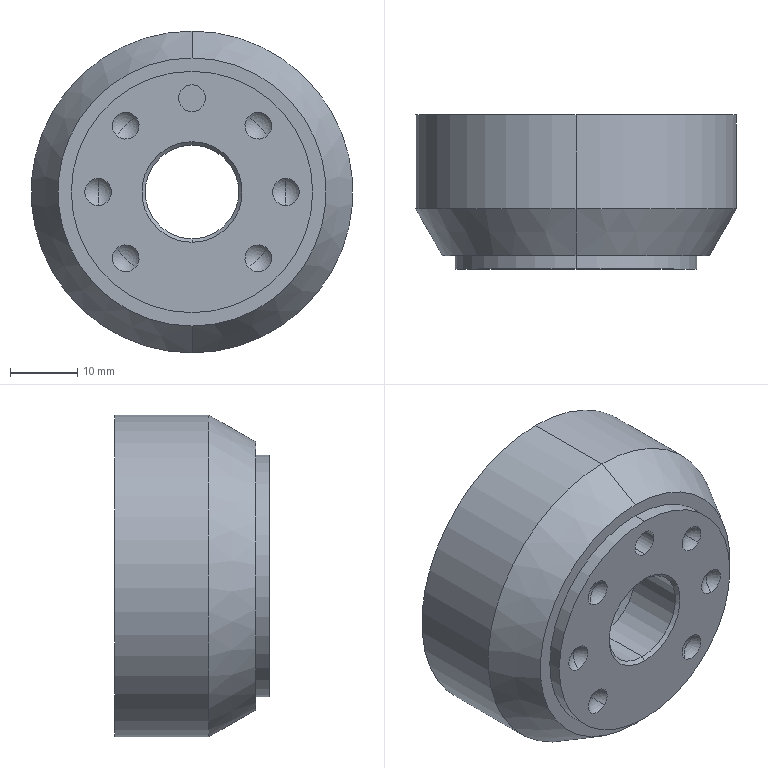Part | SolidWorks | features ICE 4, CirPattern 2, Chamfer 1, HoleWzd 1, RevCut 1, Revolution 1 | 1 solid | 58 faces | box 48 x 23 x 48 mm | volume 22097 mm3 | cone 20 | cylinder 20 | torus 12 | plane 6 | commonest cylinder face diameters 3.3 x8 4 x2 14 x2 18 x2 35 x2 36 x2
STEP:
#1=CARTESIAN_POINT('',(0.,0.5,7.));
#2=VERTEX_POINT('',#1);
#3=CARTESIAN_POINT('',(0.,0.5,-7.));
#4=VERTEX_POINT('',#3);
#5=CARTESIAN_POINT('',(0.,0.5,0.));
#6=DIRECTION('',(0.,-1.,0.));
#7=DIRECTION('',(0.,0.,-1.));
#8=AXIS2_PLACEMENT_3D('',#5,#6,#7);
#9=CIRCLE('',#8,7.);
#10=EDGE_CURVE('',#2,#4,#9,.T.);
#11=ORIENTED_EDGE('',*,*,#10,.F.);
#12=CARTESIAN_POINT('',(0.,0.,7.5));
#13=VERTEX_POINT('',#12);
#14=CARTESIAN_POINT('',(0.,0.,7.5));
#15=DIRECTION('',(0.,-0.7071,0.7071));
#16=VECTOR('',#15,1000.);
#17=LINE('',#14,#16);
#18=EDGE_CURVE('',#2,#13,#17,.T.);
#19=ORIENTED_EDGE('',*,*,#18,.T.);
#20=CARTESIAN_POINT('',(0.,0.,-7.5));
#21=VERTEX_POINT('',#20);
#22=CARTESIAN_POINT('',(0.,0.,0.));
#23=DIRECTION('',(0.,1.,0.));
#24=DIRECTION('',(0.,0.,-1.));
#25=AXIS2_PLACEMENT_3D('',#22,#23,#24);
#26=CIRCLE('',#25,7.5);
#27=EDGE_CURVE('',#21,#13,#26,.T.);
#28=ORIENTED_EDGE('',*,*,#27,.F.);
#29=CARTESIAN_POINT('',(0.,0.,-7.5));
#30=DIRECTION('',(0.,-0.7071,-0.7071));
#31=VECTOR('',#30,1000.);
#32=LINE('',#29,#31);
#33=EDGE_CURVE('',#4,#21,#32,.T.);
#34=ORIENTED_EDGE('',*,*,#33,.F.);
#35=EDGE_LOOP('',(#11,#19,#28,#34));
#36=FACE_OUTER_BOUND('',#35,.T.);
#37=CARTESIAN_POINT('',(0.,0.,0.));
#38=DIRECTION('',(0.,-1.,0.));
#39=DIRECTION('',(0.,0.,-1.));
#40=AXIS2_PLACEMENT_3D('',#37,#38,#39);
#41=CONICAL_SURFACE('',#40,7.5,0.7854);
#42=ADVANCED_FACE('',(#36),#41,.F.);
#43=CARTESIAN_POINT('',(20.75,22.625,-1.65));
#44=VERTEX_POINT('',#43);
#45=CARTESIAN_POINT('',(20.75,22.625,1.65));
#46=VERTEX_POINT('',#45);
#47=CARTESIAN_POINT('',(20.75,22.625,0.));
#48=DIRECTION('',(0.,1.,0.));
#49=DIRECTION('',(0.,0.,1.));
#50=AXIS2_PLACEMENT_3D('',#47,#48,#49);
#51=CIRCLE('',#50,1.65);
#52=EDGE_CURVE('',#44,#46,#51,.T.);
#53=ORIENTED_EDGE('',*,*,#52,.F.);
#54=CARTESIAN_POINT('',(20.75,23.,-2.025));
#55=VERTEX_POINT('',#54);
#56=CARTESIAN_POINT('',(20.75,23.,-2.025));
#57=DIRECTION('',(0.,0.7071,-0.7071));
#58=VECTOR('',#57,1000.);
#59=LINE('',#56,#58);
#60=EDGE_CURVE('',#44,#55,#59,.T.);
#61=ORIENTED_EDGE('',*,*,#60,.T.);
#62=CARTESIAN_POINT('',(20.75,23.,2.025));
#63=VERTEX_POINT('',#62);
#64=CARTESIAN_POINT('',(20.75,23.,0.));
#65=DIRECTION('',(0.,1.,0.));
#66=DIRECTION('',(0.,0.,1.));
#67=AXIS2_PLACEMENT_3D('',#64,#65,#66);
#68=CIRCLE('',#67,2.025);
#69=EDGE_CURVE('',#55,#63,#68,.T.);
#70=ORIENTED_EDGE('',*,*,#69,.T.);
#71=CARTESIAN_POINT('',(20.75,23.,2.025));
#72=DIRECTION('',(0.,0.7071,0.7071));
#73=VECTOR('',#72,1000.);
#74=LINE('',#71,#73);
#75=EDGE_CURVE('',#46,#63,#74,.T.);
#76=ORIENTED_EDGE('',*,*,#75,.F.);
#77=EDGE_LOOP('',(#53,#61,#70,#76));
#78=FACE_OUTER_BOUND('',#77,.T.);
#79=CARTESIAN_POINT('',(20.75,23.,0.));
#80=DIRECTION('',(0.,1.,0.));
#81=DIRECTION('',(0.,0.,1.));
#82=AXIS2_PLACEMENT_3D('',#79,#80,#81);
#83=CONICAL_SURFACE('',#82,2.025,0.7854);
#84=ADVANCED_FACE('',(#78),#83,.F.);
#85=CARTESIAN_POINT('',(20.75,15.,-1.65));
#86=VERTEX_POINT('',#85);
#87=CARTESIAN_POINT('',(20.75,15.,1.65));
#88=VERTEX_POINT('',#87);
#89=CARTESIAN_POINT('',(20.75,15.,0.));
#90=DIRECTION('',(0.,1.,0.));
#91=DIRECTION('',(0.,0.,1.));
#92=AXIS2_PLACEMENT_3D('',#89,#90,#91);
#93=CIRCLE('',#92,1.65);
#94=EDGE_CURVE('',#86,#88,#93,.T.);
#95=ORIENTED_EDGE('',*,*,#94,.F.);
#96=CARTESIAN_POINT('',(20.75,23.,-1.65));
#97=DIRECTION('',(0.,1.,0.));
#98=VECTOR('',#97,1000.);
#99=LINE('',#96,#98);
#100=EDGE_CURVE('',#86,#44,#99,.T.);
#101=ORIENTED_EDGE('',*,*,#100,.T.);
#102=ORIENTED_EDGE('',*,*,#52,.T.);
#103=CARTESIAN_POINT('',(20.75,23.,1.65));
#104=DIRECTION('',(0.,1.,0.));
#105=VECTOR('',#104,1000.);
#106=LINE('',#103,#105);
#107=EDGE_CURVE('',#88,#46,#106,.T.);
#108=ORIENTED_EDGE('',*,*,#107,.F.);
#109=EDGE_LOOP('',(#95,#101,#102,#108));
#110=FACE_OUTER_BOUND('',#109,.T.);
#111=CARTESIAN_POINT('',(20.75,23.,0.));
#112=DIRECTION('',(0.,1.,0.));
#113=DIRECTION('',(0.,0.,1.));
#114=AXIS2_PLACEMENT_3D('',#111,#112,#113);
#115=CYLINDRICAL_SURFACE('',#114,1.65);
#116=ADVANCED_FACE('',(#110),#115,.F.);
#117=CARTESIAN_POINT('',(20.75,14.009,0.));
#118=VERTEX_POINT('',#117);
#119=CARTESIAN_POINT('',(20.75,15.,1.65));
#120=DIRECTION('',(0.,0.515,0.8572));
#121=VECTOR('',#120,1000.);
#122=LINE('',#119,#121);
#123=EDGE_CURVE('',#118,#88,#122,.T.);
#124=ORIENTED_EDGE('',*,*,#123,.F.);
#125=CARTESIAN_POINT('',(20.75,15.,-1.65));
#126=DIRECTION('',(0.,0.515,-0.8572));
#127=VECTOR('',#126,1000.);
#128=LINE('',#125,#127);
#129=EDGE_CURVE('',#118,#86,#128,.T.);
#130=ORIENTED_EDGE('',*,*,#129,.T.);
#131=ORIENTED_EDGE('',*,*,#94,.T.);
#132=EDGE_LOOP('',(#124,#130,#131));
#133=FACE_OUTER_BOUND('',#132,.T.);
#134=CARTESIAN_POINT('',(20.75,15.,0.));
#135=DIRECTION('',(0.,1.,0.));
#136=DIRECTION('',(0.,0.,1.));
#137=AXIS2_PLACEMENT_3D('',#134,#135,#136);
#138=CONICAL_SURFACE('',#137,1.65,1.03);
#139=ADVANCED_FACE('',(#133),#138,.F.);
#140=CARTESIAN_POINT('',(0.,22.625,19.1));
#141=VERTEX_POINT('',#140);
#142=CARTESIAN_POINT('',(0.,22.625,22.4));
#143=VERTEX_POINT('',#142);
#144=CARTESIAN_POINT('',(0.,22.625,20.75));
#145=DIRECTION('',(0.,1.,0.));
#146=DIRECTION('',(0.,0.,1.));
#147=AXIS2_PLACEMENT_3D('',#144,#145,#146);
#148=CIRCLE('',#147,1.65);
#149=EDGE_CURVE('',#141,#143,#148,.T.);
#150=ORIENTED_EDGE('',*,*,#149,.F.);
#151=CARTESIAN_POINT('',(0.,23.,18.725));
#152=VERTEX_POINT('',#151);
#153=CARTESIAN_POINT('',(0.,23.,18.725));
#154=DIRECTION('',(0.,0.7071,-0.7071));
#155=VECTOR('',#154,1000.);
#156=LINE('',#153,#155);
#157=EDGE_CURVE('',#141,#152,#156,.T.);
#158=ORIENTED_EDGE('',*,*,#157,.T.);
#159=CARTESIAN_POINT('',(0.,23.,22.775));
#160=VERTEX_POINT('',#159);
#161=CARTESIAN_POINT('',(0.,23.,20.75));
#162=DIRECTION('',(0.,1.,0.));
#163=DIRECTION('',(0.,0.,1.));
#164=AXIS2_PLACEMENT_3D('',#161,#162,#163);
#165=CIRCLE('',#164,2.025);
#166=EDGE_CURVE('',#152,#160,#165,.T.);
#167=ORIENTED_EDGE('',*,*,#166,.T.);
#168=CARTESIAN_POINT('',(0.,23.,22.775));
#169=DIRECTION('',(0.,0.7071,0.7071));
#170=VECTOR('',#169,1000.);
#171=LINE('',#168,#170);
#172=EDGE_CURVE('',#143,#160,#171,.T.);
#173=ORIENTED_EDGE('',*,*,#172,.F.);
#174=EDGE_LOOP('',(#150,#158,#167,#173));
#175=FACE_OUTER_BOUND('',#174,.T.);
#176=CARTESIAN_POINT('',(0.,23.,20.75));
#177=DIRECTION('',(0.,1.,0.));
#178=DIRECTION('',(0.,0.,1.));
#179=AXIS2_PLACEMENT_3D('',#176,#177,#178);
#180=CONICAL_SURFACE('',#179,2.025,0.7854);
#181=ADVANCED_FACE('',(#175),#180,.F.);
#182=CARTESIAN_POINT('',(0.,15.,19.1));
#183=VERTEX_POINT('',#182);
#184=CARTESIAN_POINT('',(0.,15.,22.4));
#185=VERTEX_POINT('',#184);
#186=CARTESIAN_POINT('',(0.,15.,20.75));
#187=DIRECTION('',(0.,1.,0.));
#188=DIRECTION('',(0.,0.,1.));
#189=AXIS2_PLACEMENT_3D('',#186,#187,#188);
#190=CIRCLE('',#189,1.65);
#191=EDGE_CURVE('',#183,#185,#190,.T.);
#192=ORIENTED_EDGE('',*,*,#191,.F.);
#193=CARTESIAN_POINT('',(0.,23.,19.1));
#194=DIRECTION('',(0.,1.,0.));
#195=VECTOR('',#194,1000.);
#196=LINE('',#193,#195);
#197=EDGE_CURVE('',#183,#141,#196,.T.);
#198=ORIENTED_EDGE('',*,*,#197,.T.);
#199=ORIENTED_EDGE('',*,*,#149,.T.);
#200=CARTESIAN_POINT('',(0.,23.,22.4));
#201=DIRECTION('',(0.,1.,0.));
#202=VECTOR('',#201,1000.);
#203=LINE('',#200,#202);
#204=EDGE_CURVE('',#185,#143,#203,.T.);
#205=ORIENTED_EDGE('',*,*,#204,.F.);
#206=EDGE_LOOP('',(#192,#198,#199,#205));
#207=FACE_OUTER_BOUND('',#206,.T.);
#208=CARTESIAN_POINT('',(0.,23.,20.75));
#209=DIRECTION('',(0.,1.,0.));
#210=DIRECTION('',(0.,0.,1.));
#211=AXIS2_PLACEMENT_3D('',#208,#209,#210);
#212=CYLINDRICAL_SURFACE('',#211,1.65);
#213=ADVANCED_FACE('',(#207),#212,.F.);
#214=CARTESIAN_POINT('',(0.,14.009,20.75));
#215=VERTEX_POINT('',#214);
#216=CARTESIAN_POINT('',(0.,15.,22.4));
#217=DIRECTION('',(0.,0.515,0.8572));
#218=VECTOR('',#217,1000.);
#219=LINE('',#216,#218);
#220=EDGE_CURVE('',#215,#185,#219,.T.);
#221=ORIENTED_EDGE('',*,*,#220,.F.);
#222=CARTESIAN_POINT('',(0.,15.,19.1));
#223=DIRECTION('',(0.,0.515,-0.8572));
#224=VECTOR('',#223,1000.);
#225=LINE('',#222,#224);
#226=EDGE_CURVE('',#215,#183,#225,.T.);
#227=ORIENTED_EDGE('',*,*,#226,.T.);
#228=ORIENTED_EDGE('',*,*,#191,.T.);
#229=EDGE_LOOP('',(#221,#227,#228));
#230=FACE_OUTER_BOUND('',#229,.T.);
#231=CARTESIAN_POINT('',(0.,15.,20.75));
#232=DIRECTION('',(0.,1.,0.));
#233=DIRECTION('',(0.,0.,1.));
#234=AXIS2_PLACEMENT_3D('',#231,#232,#233);
#235=CONICAL_SURFACE('',#234,1.65,1.03);
#236=ADVANCED_FACE('',(#230),#235,.F.);
#237=CARTESIAN_POINT('',(-20.75,22.625,-1.65));
#238=VERTEX_POINT('',#237);
#239=CARTESIAN_POINT('',(-20.75,22.625,1.65));
#240=VERTEX_POINT('',#239);
#241=CARTESIAN_POINT('',(-20.75,22.625,0.));
#242=DIRECTION('',(0.,1.,0.));
#243=DIRECTION('',(0.,0.,1.));
#244=AXIS2_PLACEMENT_3D('',#241,#242,#243);
#245=CIRCLE('',#244,1.65);
#246=EDGE_CURVE('',#238,#240,#245,.T.);
#247=ORIENTED_EDGE('',*,*,#246,.F.);
#248=CARTESIAN_POINT('',(-20.75,23.,-2.025));
#249=VERTEX_POINT('',#248);
#250=CARTESIAN_POINT('',(-20.75,23.,-2.025));
#251=DIRECTION('',(0.,0.7071,-0.7071));
#252=VECTOR('',#251,1000.);
#253=LINE('',#250,#252);
#254=EDGE_CURVE('',#238,#249,#253,.T.);
#255=ORIENTED_EDGE('',*,*,#254,.T.);
#256=CARTESIAN_POINT('',(-20.75,23.,2.025));
#257=VERTEX_POINT('',#256);
#258=CARTESIAN_POINT('',(-20.75,23.,0.));
#259=DIRECTION('',(0.,1.,0.));
#260=DIRECTION('',(0.,0.,1.));
#261=AXIS2_PLACEMENT_3D('',#258,#259,#260);
#262=CIRCLE('',#261,2.025);
#263=EDGE_CURVE('',#249,#257,#262,.T.);
#264=ORIENTED_EDGE('',*,*,#263,.T.);
#265=CARTESIAN_POINT('',(-20.75,23.,2.025));
#266=DIRECTION('',(0.,0.7071,0.7071));
#267=VECTOR('',#266,1000.);
#268=LINE('',#265,#267);
#269=EDGE_CURVE('',#240,#257,#268,.T.);
#270=ORIENTED_EDGE('',*,*,#269,.F.);
#271=EDGE_LOOP('',(#247,#255,#264,#270));
#272=FACE_OUTER_BOUND('',#271,.T.);
#273=CARTESIAN_POINT('',(-20.75,23.,0.));
#274=DIRECTION('',(0.,1.,0.));
#275=DIRECTION('',(0.,0.,1.));
#276=AXIS2_PLACEMENT_3D('',#273,#274,#275);
#277=CONICAL_SURFACE('',#276,2.025,0.7854);
#278=ADVANCED_FACE('',(#272),#277,.F.);
#279=CARTESIAN_POINT('',(-20.75,15.,-1.65));
#280=VERTEX_POINT('',#279);
#281=CARTESIAN_POINT('',(-20.75,15.,1.65));
#282=VERTEX_POINT('',#281);
#283=CARTESIAN_POINT('',(-20.75,15.,0.));
#284=DIRECTION('',(0.,1.,0.));
#285=DIRECTION('',(0.,0.,1.));
#286=AXIS2_PLACEMENT_3D('',#283,#284,#285);
#287=CIRCLE('',#286,1.65);
#288=EDGE_CURVE('',#280,#282,#287,.T.);
#289=ORIENTED_EDGE('',*,*,#288,.F.);
#290=CARTESIAN_POINT('',(-20.75,23.,-1.65));
#291=DIRECTION('',(0.,1.,0.));
#292=VECTOR('',#291,1000.);
#293=LINE('',#290,#292);
#294=EDGE_CURVE('',#280,#238,#293,.T.);
#295=ORIENTED_EDGE('',*,*,#294,.T.);
#296=ORIENTED_EDGE('',*,*,#246,.T.);
#297=CARTESIAN_POINT('',(-20.75,23.,1.65));
#298=DIRECTION('',(0.,1.,0.));
#299=VECTOR('',#298,1000.);
#300=LINE('',#297,#299);
#301=EDGE_CURVE('',#282,#240,#300,.T.);
#302=ORIENTED_EDGE('',*,*,#301,.F.);
#303=EDGE_LOOP('',(#289,#295,#296,#302));
#304=FACE_OUTER_BOUND('',#303,.T.);
#305=CARTESIAN_POINT('',(-20.75,23.,0.));
#306=DIRECTION('',(0.,1.,0.));
#307=DIRECTION('',(0.,0.,1.));
#308=AXIS2_PLACEMENT_3D('',#305,#306,#307);
#309=CYLINDRICAL_SURFACE('',#308,1.65);
#310=ADVANCED_FACE('',(#304),#309,.F.);
#311=CARTESIAN_POINT('',(-20.75,14.009,0.));
#312=VERTEX_POINT('',#311);
#313=CARTESIAN_POINT('',(-20.75,15.,1.65));
#314=DIRECTION('',(0.,0.515,0.8572));
#315=VECTOR('',#314,1000.);
#316=LINE('',#313,#315);
#317=EDGE_CURVE('',#312,#282,#316,.T.);
#318=ORIENTED_EDGE('',*,*,#317,.F.);
#319=CARTESIAN_POINT('',(-20.75,15.,-1.65));
#320=DIRECTION('',(0.,0.515,-0.8572));
#321=VECTOR('',#320,1000.);
#322=LINE('',#319,#321);
#323=EDGE_CURVE('',#312,#280,#322,.T.);
#324=ORIENTED_EDGE('',*,*,#323,.T.);
#325=ORIENTED_EDGE('',*,*,#288,.T.);
#326=EDGE_LOOP('',(#318,#324,#325));
#327=FACE_OUTER_BOUND('',#326,.T.);
#328=CARTESIAN_POINT('',(-20.75,15.,0.));
#329=DIRECTION('',(0.,1.,0.));
#330=DIRECTION('',(0.,0.,1.));
#331=AXIS2_PLACEMENT_3D('',#328,#329,#330);
#332=CONICAL_SURFACE('',#331,1.65,1.03);
#333=ADVANCED_FACE('',(#327),#332,.F.);
#334=CARTESIAN_POINT('',(0.,22.625,-22.4));
#335=VERTEX_POINT('',#334);
#336=CARTESIAN_POINT('',(0.,22.625,-19.1));
#337=VERTEX_POINT('',#336);
#338=CARTESIAN_POINT('',(0.,22.625,-20.75));
#339=DIRECTION('',(0.,1.,0.));
#340=DIRECTION('',(0.,0.,1.));
#341=AXIS2_PLACEMENT_3D('',#338,#339,#340);
#342=CIRCLE('',#341,1.65);
#343=EDGE_CURVE('',#335,#337,#342,.T.);
#344=ORIENTED_EDGE('',*,*,#343,.F.);
#345=CARTESIAN_POINT('',(0.,23.,-22.775));
#346=VERTEX_POINT('',#345);
#347=CARTESIAN_POINT('',(0.,23.,-22.775));
#348=DIRECTION('',(0.,0.7071,-0.7071));
#349=VECTOR('',#348,1000.);
#350=LINE('',#347,#349);
#351=EDGE_CURVE('',#335,#346,#350,.T.);
#352=ORIENTED_EDGE('',*,*,#351,.T.);
#353=CARTESIAN_POINT('',(0.,23.,-18.725));
#354=VERTEX_POINT('',#353);
#355=CARTESIAN_POINT('',(0.,23.,-20.75));
#356=DIRECTION('',(0.,1.,0.));
#357=DIRECTION('',(0.,0.,1.));
#358=AXIS2_PLACEMENT_3D('',#355,#356,#357);
#359=CIRCLE('',#358,2.025);
#360=EDGE_CURVE('',#346,#354,#359,.T.);
#361=ORIENTED_EDGE('',*,*,#360,.T.);
#362=CARTESIAN_POINT('',(0.,23.,-18.725));
#363=DIRECTION('',(0.,0.7071,0.7071));
#364=VECTOR('',#363,1000.);
#365=LINE('',#362,#364);
#366=EDGE_CURVE('',#337,#354,#365,.T.);
#367=ORIENTED_EDGE('',*,*,#366,.F.);
#368=EDGE_LOOP('',(#344,#352,#361,#367));
#369=FACE_OUTER_BOUND('',#368,.T.);
#370=CARTESIAN_POINT('',(0.,23.,-20.75));
#371=DIRECTION('',(0.,1.,0.));
#372=DIRECTION('',(0.,0.,1.));
#373=AXIS2_PLACEMENT_3D('',#370,#371,#372);
#374=CONICAL_SURFACE('',#373,2.025,0.7854);
#375=ADVANCED_FACE('',(#369),#374,.F.);
#376=CARTESIAN_POINT('',(0.,15.,-22.4));
#377=VERTEX_POINT('',#376);
#378=CARTESIAN_POINT('',(0.,15.,-19.1));
#379=VERTEX_POINT('',#378);
#380=CARTESIAN_POINT('',(0.,15.,-20.75));
#381=DIRECTION('',(0.,1.,0.));
#382=DIRECTION('',(0.,0.,1.));
#383=AXIS2_PLACEMENT_3D('',#380,#381,#382);
#384=CIRCLE('',#383,1.65);
#385=EDGE_CURVE('',#377,#379,#384,.T.);
#386=ORIENTED_EDGE('',*,*,#385,.F.);
#387=CARTESIAN_POINT('',(0.,23.,-22.4));
#388=DIRECTION('',(0.,1.,0.));
#389=VECTOR('',#388,1000.);
#390=LINE('',#387,#389);
#391=EDGE_CURVE('',#377,#335,#390,.T.);
#392=ORIENTED_EDGE('',*,*,#391,.T.);
#393=ORIENTED_EDGE('',*,*,#343,.T.);
#394=CARTESIAN_POINT('',(0.,23.,-19.1));
#395=DIRECTION('',(0.,1.,0.));
#396=VECTOR('',#395,1000.);
#397=LINE('',#394,#396);
#398=EDGE_CURVE('',#379,#337,#397,.T.);
#399=ORIENTED_EDGE('',*,*,#398,.F.);
#400=EDGE_LOOP('',(#386,#392,#393,#399));
#401=FACE_OUTER_BOUND('',#400,.T.);
#402=CARTESIAN_POINT('',(0.,23.,-20.75));
#403=DIRECTION('',(0.,1.,0.));
#404=DIRECTION('',(0.,0.,1.));
#405=AXIS2_PLACEMENT_3D('',#402,#403,#404);
#406=CYLINDRICAL_SURFACE('',#405,1.65);
#407=ADVANCED_FACE('',(#401),#406,.F.);
#408=CARTESIAN_POINT('',(0.,14.009,-20.75));
#409=VERTEX_POINT('',#408);
#410=CARTESIAN_POINT('',(0.,15.,-19.1));
#411=DIRECTION('',(0.,0.515,0.8572));
#412=VECTOR('',#411,1000.);
#413=LINE('',#410,#412);
#414=EDGE_CURVE('',#409,#379,#413,.T.);
#415=ORIENTED_EDGE('',*,*,#414,.F.);
#416=CARTESIAN_POINT('',(0.,15.,-22.4));
#417=DIRECTION('',(0.,0.515,-0.8572));
#418=VECTOR('',#417,1000.);
#419=LINE('',#416,#418);
#420=EDGE_CURVE('',#409,#377,#419,.T.);
#421=ORIENTED_EDGE('',*,*,#420,.T.);
#422=ORIENTED_EDGE('',*,*,#385,.T.);
#423=EDGE_LOOP('',(#415,#421,#422));
#424=FACE_OUTER_BOUND('',#423,.T.);
#425=CARTESIAN_POINT('',(0.,15.,-20.75));
#426=DIRECTION('',(0.,1.,0.));
#427=DIRECTION('',(0.,0.,1.));
#428=AXIS2_PLACEMENT_3D('',#425,#426,#427);
#429=CONICAL_SURFACE('',#428,1.65,1.03);
#430=ADVANCED_FACE('',(#424),#429,.F.);
#431=CARTESIAN_POINT('',(-9.899,1.,-9.899));
#432=VERTEX_POINT('',#431);
#433=CARTESIAN_POINT('',(-8.485,0.,-11.314));
#434=VERTEX_POINT('',#433);
#435=CARTESIAN_POINT('',(-10.004,-1.796,-9.795));
#436=DIRECTION('',(-0.7071,0.,-0.7071));
#437=DIRECTION('',(-0.7071,0.,0.7071));
#438=AXIS2_PLACEMENT_3D('',#435,#436,#437);
#439=CIRCLE('',#438,2.8);
#440=EDGE_CURVE('',#432,#434,#439,.T.);
#441=ORIENTED_EDGE('',*,*,#440,.F.);
#442=CARTESIAN_POINT('',(-11.314,0.,-8.485));
#443=VERTEX_POINT('',#442);
#444=CARTESIAN_POINT('',(-9.795,-1.796,-10.004));
#445=DIRECTION('',(0.7071,0.,0.7071));
#446=DIRECTION('',(0.7071,0.,-0.7071));
#447=AXIS2_PLACEMENT_3D('',#444,#445,#446);
#448=CIRCLE('',#447,2.8);
#449=EDGE_CURVE('',#432,#443,#448,.T.);
#450=ORIENTED_EDGE('',*,*,#449,.T.);
#451=CARTESIAN_POINT('',(-9.899,0.,-9.899));
#452=DIRECTION('',(0.,-1.,0.));
#453=DIRECTION('',(0.7071,0.,-0.7071));
#454=AXIS2_PLACEMENT_3D('',#451,#452,#453);
#455=CIRCLE('',#454,2.);
#456=EDGE_CURVE('',#443,#434,#455,.T.);
#457=ORIENTED_EDGE('',*,*,#456,.T.);
#458=EDGE_LOOP('',(#441,#450,#457));
#459=FACE_OUTER_BOUND('',#458,.T.);
#460=CARTESIAN_POINT('',(-9.899,-1.796,-9.899));
#461=DIRECTION('',(0.,-1.,0.));
#462=DIRECTION('',(0.7071,0.,-0.7071));
#463=AXIS2_PLACEMENT_3D('',#460,#461,#462);
#464=TOROIDAL_SURFACE('',#463,-0.148,2.8);
#465=ADVANCED_FACE('',(#459),#464,.F.);
#466=CARTESIAN_POINT('',(9.899,1.,-9.899));
#467=VERTEX_POINT('',#466);
#468=CARTESIAN_POINT('',(11.314,0.,-8.485));
#469=VERTEX_POINT('',#468);
#470=CARTESIAN_POINT('',(9.795,-1.796,-10.004));
#471=DIRECTION('',(0.7071,0.,-0.7071));
#472=DIRECTION('',(-0.7071,0.,-0.7071));
#473=AXIS2_PLACEMENT_3D('',#470,#471,#472);
#474=CIRCLE('',#473,2.8);
#475=EDGE_CURVE('',#467,#469,#474,.T.);
#476=ORIENTED_EDGE('',*,*,#475,.F.);
#477=CARTESIAN_POINT('',(8.485,0.,-11.314));
#478=VERTEX_POINT('',#477);
#479=CARTESIAN_POINT('',(10.004,-1.796,-9.795));
#480=DIRECTION('',(-0.7071,0.,0.7071));
#481=DIRECTION('',(0.7071,0.,0.7071));
#482=AXIS2_PLACEMENT_3D('',#479,#480,#481);
#483=CIRCLE('',#482,2.8);
#484=EDGE_CURVE('',#467,#478,#483,.T.);
#485=ORIENTED_EDGE('',*,*,#484,.T.);
#486=CARTESIAN_POINT('',(9.899,0.,-9.899));
#487=DIRECTION('',(0.,-1.,0.));
#488=DIRECTION('',(0.7071,0.,0.7071));
#489=AXIS2_PLACEMENT_3D('',#486,#487,#488);
#490=CIRCLE('',#489,2.);
#491=EDGE_CURVE('',#478,#469,#490,.T.);
#492=ORIENTED_EDGE('',*,*,#491,.T.);
#493=EDGE_LOOP('',(#476,#485,#492));
#494=FACE_OUTER_BOUND('',#493,.T.);
#495=CARTESIAN_POINT('',(9.899,-1.796,-9.899));
#496=DIRECTION('',(0.,-1.,0.));
#497=DIRECTION('',(0.7071,0.,0.7071));
#498=AXIS2_PLACEMENT_3D('',#495,#496,#497);
#499=TOROIDAL_SURFACE('',#498,-0.148,2.8);
#500=ADVANCED_FACE('',(#494),#499,.F.);
#501=CARTESIAN_POINT('',(14.,1.,0.));
#502=VERTEX_POINT('',#501);
#503=CARTESIAN_POINT('',(14.,0.,2.));
#504=VERTEX_POINT('',#503);
#505=CARTESIAN_POINT('',(14.,-1.796,-0.148));
#506=DIRECTION('',(1.,0.,0.));
#507=DIRECTION('',(0.,0.,-1.));
#508=AXIS2_PLACEMENT_3D('',#505,#506,#507);
#509=CIRCLE('',#508,2.8);
#510=EDGE_CURVE('',#502,#504,#509,.T.);
#511=ORIENTED_EDGE('',*,*,#510,.F.);
#512=CARTESIAN_POINT('',(14.,0.,-2.));
#513=VERTEX_POINT('',#512);
#514=CARTESIAN_POINT('',(14.,-1.796,0.148));
#515=DIRECTION('',(-1.,0.,0.));
#516=DIRECTION('',(0.,0.,1.));
#517=AXIS2_PLACEMENT_3D('',#514,#515,#516);
#518=CIRCLE('',#517,2.8);
#519=EDGE_CURVE('',#502,#513,#518,.T.);
#520=ORIENTED_EDGE('',*,*,#519,.T.);
#521=CARTESIAN_POINT('',(14.,0.,0.));
#522=DIRECTION('',(0.,-1.,0.));
#523=DIRECTION('',(0.,0.,1.));
#524=AXIS2_PLACEMENT_3D('',#521,#522,#523);
#525=CIRCLE('',#524,2.);
#526=EDGE_CURVE('',#513,#504,#525,.T.);
#527=ORIENTED_EDGE('',*,*,#526,.T.);
#528=EDGE_LOOP('',(#511,#520,#527));
#529=FACE_OUTER_BOUND('',#528,.T.);
#530=CARTESIAN_POINT('',(14.,-1.796,0.));
#531=DIRECTION('',(0.,-1.,0.));
#532=DIRECTION('',(0.,0.,1.));
#533=AXIS2_PLACEMENT_3D('',#530,#531,#532);
#534=TOROIDAL_SURFACE('',#533,-0.148,2.8);
#535=ADVANCED_FACE('',(#529),#534,.F.);
#536=CARTESIAN_POINT('',(9.899,1.,9.899));
#537=VERTEX_POINT('',#536);
#538=CARTESIAN_POINT('',(8.485,0.,11.314));
#539=VERTEX_POINT('',#538);
#540=CARTESIAN_POINT('',(10.004,-1.796,9.795));
#541=DIRECTION('',(0.7071,0.,0.7071));
#542=DIRECTION('',(0.7071,0.,-0.7071));
#543=AXIS2_PLACEMENT_3D('',#540,#541,#542);
#544=CIRCLE('',#543,2.8);
#545=EDGE_CURVE('',#537,#539,#544,.T.);
#546=ORIENTED_EDGE('',*,*,#545,.F.);
#547=CARTESIAN_POINT('',(11.314,0.,8.485));
#548=VERTEX_POINT('',#547);
#549=CARTESIAN_POINT('',(9.795,-1.796,10.004));
#550=DIRECTION('',(-0.7071,0.,-0.7071));
#551=DIRECTION('',(-0.7071,0.,0.7071));
#552=AXIS2_PLACEMENT_3D('',#549,#550,#551);
#553=CIRCLE('',#552,2.8);
#554=EDGE_CURVE('',#537,#548,#553,.T.);
#555=ORIENTED_EDGE('',*,*,#554,.T.);
#556=CARTESIAN_POINT('',(9.899,0.,9.899));
#557=DIRECTION('',(0.,-1.,0.));
#558=DIRECTION('',(-0.7071,0.,0.7071));
#559=AXIS2_PLACEMENT_3D('',#556,#557,#558);
#560=CIRCLE('',#559,2.);
#561=EDGE_CURVE('',#548,#539,#560,.T.);
#562=ORIENTED_EDGE('',*,*,#561,.T.);
#563=EDGE_LOOP('',(#546,#555,#562));
#564=FACE_OUTER_BOUND('',#563,.T.);
#565=CARTESIAN_POINT('',(9.899,-1.796,9.899));
#566=DIRECTION('',(0.,-1.,0.));
#567=DIRECTION('',(-0.7071,0.,0.7071));
#568=AXIS2_PLACEMENT_3D('',#565,#566,#567);
#569=TOROIDAL_SURFACE('',#568,-0.148,2.8);
#570=ADVANCED_FACE('',(#564),#569,.F.);
#571=CARTESIAN_POINT('',(-9.899,1.,9.899));
#572=VERTEX_POINT('',#571);
#573=CARTESIAN_POINT('',(-11.314,0.,8.485));
#574=VERTEX_POINT('',#573);
#575=CARTESIAN_POINT('',(-9.795,-1.796,10.004));
#576=DIRECTION('',(-0.7071,0.,0.7071));
#577=DIRECTION('',(0.7071,0.,0.7071));
#578=AXIS2_PLACEMENT_3D('',#575,#576,#577);
#579=CIRCLE('',#578,2.8);
#580=EDGE_CURVE('',#572,#574,#579,.T.);
#581=ORIENTED_EDGE('',*,*,#580,.F.);
#582=CARTESIAN_POINT('',(-8.485,0.,11.314));
#583=VERTEX_POINT('',#582);
#584=CARTESIAN_POINT('',(-10.004,-1.796,9.795));
#585=DIRECTION('',(0.7071,0.,-0.7071));
#586=DIRECTION('',(-0.7071,0.,-0.7071));
#587=AXIS2_PLACEMENT_3D('',#584,#585,#586);
#588=CIRCLE('',#587,2.8);
#589=EDGE_CURVE('',#572,#583,#588,.T.);
#590=ORIENTED_EDGE('',*,*,#589,.T.);
#591=CARTESIAN_POINT('',(-9.899,0.,9.899));
#592=DIRECTION('',(0.,-1.,0.));
#593=DIRECTION('',(-0.7071,0.,-0.7071));
#594=AXIS2_PLACEMENT_3D('',#591,#592,#593);
#595=CIRCLE('',#594,2.);
#596=EDGE_CURVE('',#583,#574,#595,.T.);
#597=ORIENTED_EDGE('',*,*,#596,.T.);
#598=EDGE_LOOP('',(#581,#590,#597));
#599=FACE_OUTER_BOUND('',#598,.T.);
#600=CARTESIAN_POINT('',(-9.899,-1.796,9.899));
#601=DIRECTION('',(0.,-1.,0.));
#602=DIRECTION('',(-0.7071,0.,-0.7071));
#603=AXIS2_PLACEMENT_3D('',#600,#601,#602);
#604=TOROIDAL_SURFACE('',#603,-0.148,2.8);
#605=ADVANCED_FACE('',(#599),#604,.F.);
#606=CARTESIAN_POINT('',(-14.,1.,0.));
#607=VERTEX_POINT('',#606);
#608=CARTESIAN_POINT('',(-14.,0.,-2.));
#609=VERTEX_POINT('',#608);
#610=CARTESIAN_POINT('',(-14.,-1.796,0.148));
#611=DIRECTION('',(-1.,0.,0.));
#612=DIRECTION('',(0.,0.,1.));
#613=AXIS2_PLACEMENT_3D('',#610,#611,#612);
#614=CIRCLE('',#613,2.8);
#615=EDGE_CURVE('',#607,#609,#614,.T.);
#616=ORIENTED_EDGE('',*,*,#615,.F.);
#617=CARTESIAN_POINT('',(-14.,0.,2.));
#618=VERTEX_POINT('',#617);
#619=CARTESIAN_POINT('',(-14.,-1.796,-0.148));
#620=DIRECTION('',(1.,0.,0.));
#621=DIRECTION('',(0.,0.,-1.));
#622=AXIS2_PLACEMENT_3D('',#619,#620,#621);
#623=CIRCLE('',#622,2.8);
#624=EDGE_CURVE('',#607,#618,#623,.T.);
#625=ORIENTED_EDGE('',*,*,#624,.T.);
#626=CARTESIAN_POINT('',(-14.,0.,0.));
#627=DIRECTION('',(0.,-1.,0.));
#628=DIRECTION('',(0.,0.,-1.));
#629=AXIS2_PLACEMENT_3D('',#626,#627,#628);
#630=CIRCLE('',#629,2.);
#631=EDGE_CURVE('',#618,#609,#630,.T.);
#632=ORIENTED_EDGE('',*,*,#631,.T.);
#633=EDGE_LOOP('',(#616,#625,#632));
#634=FACE_OUTER_BOUND('',#633,.T.);
#635=CARTESIAN_POINT('',(-14.,-1.796,0.));
#636=DIRECTION('',(0.,-1.,0.));
#637=DIRECTION('',(0.,0.,-1.));
#638=AXIS2_PLACEMENT_3D('',#635,#636,#637);
#639=TOROIDAL_SURFACE('',#638,-0.148,2.8);
#640=ADVANCED_FACE('',(#634),#639,.F.);
#641=CARTESIAN_POINT('',(0.,4.,16.));
#642=VERTEX_POINT('',#641);
#643=CARTESIAN_POINT('',(0.,4.,12.));
#644=VERTEX_POINT('',#643);
#645=CARTESIAN_POINT('',(0.,4.,14.));
#646=DIRECTION('',(0.,-1.,0.));
#647=DIRECTION('',(0.,0.,-1.));
#648=AXIS2_PLACEMENT_3D('',#645,#646,#647);
#649=CIRCLE('',#648,2.);
#650=EDGE_CURVE('',#642,#644,#649,.T.);
#651=ORIENTED_EDGE('',*,*,#650,.F.);
#652=CARTESIAN_POINT('',(0.,0.,16.));
#653=VERTEX_POINT('',#652);
#654=CARTESIAN_POINT('',(0.,4.,16.));
#655=DIRECTION('',(0.,-1.,0.));
#656=VECTOR('',#655,1000.);
#657=LINE('',#654,#656);
#658=EDGE_CURVE('',#642,#653,#657,.T.);
#659=ORIENTED_EDGE('',*,*,#658,.T.);
#660=CARTESIAN_POINT('',(0.,0.,12.));
#661=VERTEX_POINT('',#660);
#662=CARTESIAN_POINT('',(0.,0.,14.));
#663=DIRECTION('',(0.,-1.,0.));
#664=DIRECTION('',(0.,0.,-1.));
#665=AXIS2_PLACEMENT_3D('',#662,#663,#664);
#666=CIRCLE('',#665,2.);
#667=EDGE_CURVE('',#653,#661,#666,.T.);
#668=ORIENTED_EDGE('',*,*,#667,.T.);
#669=CARTESIAN_POINT('',(0.,4.,12.));
#670=DIRECTION('',(0.,-1.,0.));
#671=VECTOR('',#670,1000.);
#672=LINE('',#669,#671);
#673=EDGE_CURVE('',#644,#661,#672,.T.);
#674=ORIENTED_EDGE('',*,*,#673,.F.);
#675=EDGE_LOOP('',(#651,#659,#668,#674));
#676=FACE_OUTER_BOUND('',#675,.T.);
#677=CARTESIAN_POINT('',(0.,4.,14.));
#678=DIRECTION('',(0.,-1.,0.));
#679=DIRECTION('',(0.,0.,-1.));
#680=AXIS2_PLACEMENT_3D('',#677,#678,#679);
#681=CYLINDRICAL_SURFACE('',#680,2.);
#682=ADVANCED_FACE('',(#676),#681,.F.);
#683=ORIENTED_EDGE('',*,*,#10,.T.);
#684=CARTESIAN_POINT('',(0.,9.,-7.));
#685=VERTEX_POINT('',#684);
#686=CARTESIAN_POINT('',(0.,0.,-7.));
#687=DIRECTION('',(0.,1.,0.));
#688=VECTOR('',#687,1000.);
#689=LINE('',#686,#688);
#690=EDGE_CURVE('',#4,#685,#689,.T.);
#691=ORIENTED_EDGE('',*,*,#690,.T.);
#692=CARTESIAN_POINT('',(0.,9.,7.));
#693=VERTEX_POINT('',#692);
#694=CARTESIAN_POINT('',(0.,9.,0.));
#695=DIRECTION('',(0.,1.,0.));
#696=DIRECTION('',(0.,0.,1.));
#697=AXIS2_PLACEMENT_3D('',#694,#695,#696);
#698=CIRCLE('',#697,7.);
#699=EDGE_CURVE('',#685,#693,#698,.T.);
#700=ORIENTED_EDGE('',*,*,#699,.T.);
#701=CARTESIAN_POINT('',(0.,0.,7.));
#702=DIRECTION('',(0.,1.,0.));
#703=VECTOR('',#702,1000.);
#704=LINE('',#701,#703);
#705=EDGE_CURVE('',#2,#693,#704,.T.);
#706=ORIENTED_EDGE('',*,*,#705,.F.);
#707=EDGE_LOOP('',(#683,#691,#700,#706));
#708=FACE_OUTER_BOUND('',#707,.T.);
#709=CARTESIAN_POINT('',(0.,0.,0.));
#710=DIRECTION('',(0.,1.,0.));
#711=DIRECTION('',(0.,0.,1.));
#712=AXIS2_PLACEMENT_3D('',#709,#710,#711);
#713=CYLINDRICAL_SURFACE('',#712,7.);
#714=ADVANCED_FACE('',(#708),#713,.F.);
#715=CARTESIAN_POINT('',(0.,9.,9.));
#716=VERTEX_POINT('',#715);
#717=CARTESIAN_POINT('',(0.,9.,-9.));
#718=VERTEX_POINT('',#717);
#719=CARTESIAN_POINT('',(0.,9.,0.));
#720=DIRECTION('',(0.,1.,0.));
#721=DIRECTION('',(0.,0.,1.));
#722=AXIS2_PLACEMENT_3D('',#719,#720,#721);
#723=CIRCLE('',#722,9.);
#724=EDGE_CURVE('',#716,#718,#723,.T.);
#725=ORIENTED_EDGE('',*,*,#724,.F.);
#726=CARTESIAN_POINT('',(0.,8.,9.));
#727=VERTEX_POINT('',#726);
#728=CARTESIAN_POINT('',(0.,9.,9.));
#729=DIRECTION('',(0.,-1.,0.));
#730=VECTOR('',#729,1000.);
#731=LINE('',#728,#730);
#732=EDGE_CURVE('',#716,#727,#731,.T.);
#733=ORIENTED_EDGE('',*,*,#732,.T.);
#734=CARTESIAN_POINT('',(0.,8.,-9.));
#735=VERTEX_POINT('',#734);
#736=CARTESIAN_POINT('',(0.,8.,0.));
#737=DIRECTION('',(0.,1.,0.));
#738=DIRECTION('',(0.,0.,1.));
#739=AXIS2_PLACEMENT_3D('',#736,#737,#738);
#740=CIRCLE('',#739,9.);
#741=EDGE_CURVE('',#727,#735,#740,.T.);
#742=ORIENTED_EDGE('',*,*,#741,.T.);
#743=CARTESIAN_POINT('',(0.,9.,-9.));
#744=DIRECTION('',(0.,-1.,0.));
#745=VECTOR('',#744,1000.);
#746=LINE('',#743,#745);
#747=EDGE_CURVE('',#718,#735,#746,.T.);
#748=ORIENTED_EDGE('',*,*,#747,.F.);
#749=EDGE_LOOP('',(#725,#733,#742,#748));
#750=FACE_OUTER_BOUND('',#749,.T.);
#751=CARTESIAN_POINT('',(0.,9.,0.));
#752=DIRECTION('',(0.,-1.,0.));
#753=DIRECTION('',(0.,0.,-1.));
#754=AXIS2_PLACEMENT_3D('',#751,#752,#753);
#755=CYLINDRICAL_SURFACE('',#754,9.);
#756=ADVANCED_FACE('',(#750),#755,.T.);
#757=CARTESIAN_POINT('',(0.,8.,-17.5));
#758=VERTEX_POINT('',#757);
#759=CARTESIAN_POINT('',(0.,8.,17.5));
#760=VERTEX_POINT('',#759);
#761=CARTESIAN_POINT('',(0.,8.,0.));
#762=DIRECTION('',(0.,1.,0.));
#763=DIRECTION('',(0.,0.,1.));
#764=AXIS2_PLACEMENT_3D('',#761,#762,#763);
#765=CIRCLE('',#764,17.5);
#766=EDGE_CURVE('',#758,#760,#765,.T.);
#767=ORIENTED_EDGE('',*,*,#766,.F.);
#768=CARTESIAN_POINT('',(0.,23.,-17.5));
#769=VERTEX_POINT('',#768);
#770=CARTESIAN_POINT('',(0.,8.,-17.5));
#771=DIRECTION('',(0.,1.,0.));
#772=VECTOR('',#771,1000.);
#773=LINE('',#770,#772);
#774=EDGE_CURVE('',#758,#769,#773,.T.);
#775=ORIENTED_EDGE('',*,*,#774,.T.);
#776=CARTESIAN_POINT('',(0.,23.,17.5));
#777=VERTEX_POINT('',#776);
#778=CARTESIAN_POINT('',(0.,23.,0.));
#779=DIRECTION('',(0.,1.,0.));
#780=DIRECTION('',(0.,0.,1.));
#781=AXIS2_PLACEMENT_3D('',#778,#779,#780);
#782=CIRCLE('',#781,17.5);
#783=EDGE_CURVE('',#769,#777,#782,.T.);
#784=ORIENTED_EDGE('',*,*,#783,.T.);
#785=CARTESIAN_POINT('',(0.,8.,17.5));
#786=DIRECTION('',(0.,1.,0.));
#787=VECTOR('',#786,1000.);
#788=LINE('',#785,#787);
#789=EDGE_CURVE('',#760,#777,#788,.T.);
#790=ORIENTED_EDGE('',*,*,#789,.F.);
#791=EDGE_LOOP('',(#767,#775,#784,#790));
#792=FACE_OUTER_BOUND('',#791,.T.);
#793=CARTESIAN_POINT('',(0.,8.,0.));
#794=DIRECTION('',(0.,1.,0.));
#795=DIRECTION('',(0.,0.,1.));
#796=AXIS2_PLACEMENT_3D('',#793,#794,#795);
#797=CYLINDRICAL_SURFACE('',#796,17.5);
#798=ADVANCED_FACE('',(#792),#797,.F.);
#799=CARTESIAN_POINT('',(0.,9.,24.));
#800=VERTEX_POINT('',#799);
#801=CARTESIAN_POINT('',(0.,9.,-24.));
#802=VERTEX_POINT('',#801);
#803=CARTESIAN_POINT('',(0.,9.,0.));
#804=DIRECTION('',(0.,1.,0.));
#805=DIRECTION('',(0.,0.,1.));
#806=AXIS2_PLACEMENT_3D('',#803,#804,#805);
#807=CIRCLE('',#806,24.);
#808=EDGE_CURVE('',#800,#802,#807,.T.);
#809=ORIENTED_EDGE('',*,*,#808,.T.);
#810=CARTESIAN_POINT('',(0.,23.,-24.));
#811=VERTEX_POINT('',#810);
#812=CARTESIAN_POINT('',(0.,23.,-24.));
#813=DIRECTION('',(0.,1.,0.));
#814=VECTOR('',#813,1000.);
#815=LINE('',#812,#814);
#816=EDGE_CURVE('',#802,#811,#815,.T.);
#817=ORIENTED_EDGE('',*,*,#816,.T.);
#818=CARTESIAN_POINT('',(0.,23.,24.));
#819=VERTEX_POINT('',#818);
#820=CARTESIAN_POINT('',(0.,23.,0.));
#821=DIRECTION('',(0.,1.,0.));
#822=DIRECTION('',(0.,0.,1.));
#823=AXIS2_PLACEMENT_3D('',#820,#821,#822);
#824=CIRCLE('',#823,24.);
#825=EDGE_CURVE('',#819,#811,#824,.T.);
#826=ORIENTED_EDGE('',*,*,#825,.F.);
#827=CARTESIAN_POINT('',(0.,23.,24.));
#828=DIRECTION('',(0.,1.,0.));
#829=VECTOR('',#828,1000.);
#830=LINE('',#827,#829);
#831=EDGE_CURVE('',#800,#819,#830,.T.);
#832=ORIENTED_EDGE('',*,*,#831,.F.);
#833=EDGE_LOOP('',(#809,#817,#826,#832));
#834=FACE_OUTER_BOUND('',#833,.T.);
#835=CARTESIAN_POINT('',(0.,23.,0.));
#836=DIRECTION('',(0.,1.,0.));
#837=DIRECTION('',(0.,0.,1.));
#838=AXIS2_PLACEMENT_3D('',#835,#836,#837);
#839=CYLINDRICAL_SURFACE('',#838,24.);
#840=ADVANCED_FACE('',(#834),#839,.T.);
#841=CARTESIAN_POINT('',(0.,2.,20.));
#842=VERTEX_POINT('',#841);
#843=CARTESIAN_POINT('',(0.,2.,-20.));
#844=VERTEX_POINT('',#843);
#845=CARTESIAN_POINT('',(0.,2.,0.));
#846=DIRECTION('',(0.,1.,0.));
#847=DIRECTION('',(0.,0.,1.));
#848=AXIS2_PLACEMENT_3D('',#845,#846,#847);
#849=CIRCLE('',#848,20.);
#850=EDGE_CURVE('',#842,#844,#849,.T.);
#851=ORIENTED_EDGE('',*,*,#850,.T.);
#852=CARTESIAN_POINT('',(0.,9.,-24.));
#853=DIRECTION('',(0.,0.8682,-0.4961));
#854=VECTOR('',#853,1000.);
#855=LINE('',#852,#854);
#856=EDGE_CURVE('',#844,#802,#855,.T.);
#857=ORIENTED_EDGE('',*,*,#856,.T.);
#858=ORIENTED_EDGE('',*,*,#808,.F.);
#859=CARTESIAN_POINT('',(0.,9.,24.));
#860=DIRECTION('',(0.,0.8682,0.4961));
#861=VECTOR('',#860,1000.);
#862=LINE('',#859,#861);
#863=EDGE_CURVE('',#842,#800,#862,.T.);
#864=ORIENTED_EDGE('',*,*,#863,.F.);
#865=EDGE_LOOP('',(#851,#857,#858,#864));
#866=FACE_OUTER_BOUND('',#865,.T.);
#867=CARTESIAN_POINT('',(0.,9.,0.));
#868=DIRECTION('',(0.,1.,0.));
#869=DIRECTION('',(0.,0.,1.));
#870=AXIS2_PLACEMENT_3D('',#867,#868,#869);
#871=CONICAL_SURFACE('',#870,24.,0.5191);
#872=ADVANCED_FACE('',(#866),#871,.T.);
#873=CARTESIAN_POINT('',(0.,0.,18.));
#874=VERTEX_POINT('',#873);
#875=CARTESIAN_POINT('',(0.,0.,-18.));
#876=VERTEX_POINT('',#875);
#877=CARTESIAN_POINT('',(0.,0.,0.));
#878=DIRECTION('',(0.,1.,0.));
#879=DIRECTION('',(0.,0.,1.));
#880=AXIS2_PLACEMENT_3D('',#877,#878,#879);
#881=CIRCLE('',#880,18.);
#882=EDGE_CURVE('',#874,#876,#881,.T.);
#883=ORIENTED_EDGE('',*,*,#882,.T.);
#884=CARTESIAN_POINT('',(0.,2.,-18.));
#885=VERTEX_POINT('',#884);
#886=CARTESIAN_POINT('',(0.,23.,-18.));
#887=DIRECTION('',(0.,1.,0.));
#888=VECTOR('',#887,1000.);
#889=LINE('',#886,#888);
#890=EDGE_CURVE('',#876,#885,#889,.T.);
#891=ORIENTED_EDGE('',*,*,#890,.T.);
#892=CARTESIAN_POINT('',(0.,2.,18.));
#893=VERTEX_POINT('',#892);
#894=CARTESIAN_POINT('',(0.,2.,0.));
#895=DIRECTION('',(0.,1.,0.));
#896=DIRECTION('',(0.,0.,1.));
#897=AXIS2_PLACEMENT_3D('',#894,#895,#896);
#898=CIRCLE('',#897,18.);
#899=EDGE_CURVE('',#893,#885,#898,.T.);
#900=ORIENTED_EDGE('',*,*,#899,.F.);
#901=CARTESIAN_POINT('',(0.,23.,18.));
#902=DIRECTION('',(0.,1.,0.));
#903=VECTOR('',#902,1000.);
#904=LINE('',#901,#903);
#905=EDGE_CURVE('',#874,#893,#904,.T.);
#906=ORIENTED_EDGE('',*,*,#905,.F.);
#907=EDGE_LOOP('',(#883,#891,#900,#906));
#908=FACE_OUTER_BOUND('',#907,.T.);
#909=CARTESIAN_POINT('',(0.,23.,0.));
#910=DIRECTION('',(0.,1.,0.));
#911=DIRECTION('',(0.,0.,1.));
#912=AXIS2_PLACEMENT_3D('',#909,#910,#911);
#913=CYLINDRICAL_SURFACE('',#912,18.);
#914=ADVANCED_FACE('',(#908),#913,.T.);
#915=ORIENTED_EDGE('',*,*,#27,.T.);
#916=CARTESIAN_POINT('',(0.,0.,0.));
#917=DIRECTION('',(0.,1.,0.));
#918=DIRECTION('',(0.,0.,-1.));
#919=AXIS2_PLACEMENT_3D('',#916,#917,#918);
#920=CIRCLE('',#919,7.5);
#921=EDGE_CURVE('',#13,#21,#920,.T.);
#922=ORIENTED_EDGE('',*,*,#921,.T.);
#923=EDGE_LOOP('',(#915,#922));
#924=FACE_BOUND('',#923,.T.);
#925=CARTESIAN_POINT('',(-9.899,0.,-9.899));
#926=DIRECTION('',(0.,-1.,0.));
#927=DIRECTION('',(0.7071,0.,-0.7071));
#928=AXIS2_PLACEMENT_3D('',#925,#926,#927);
#929=CIRCLE('',#928,2.);
#930=EDGE_CURVE('',#434,#443,#929,.T.);
#931=ORIENTED_EDGE('',*,*,#930,.F.);
#932=ORIENTED_EDGE('',*,*,#456,.F.);
#933=EDGE_LOOP('',(#931,#932));
#934=FACE_BOUND('',#933,.T.);
#935=CARTESIAN_POINT('',(9.899,0.,-9.899));
#936=DIRECTION('',(0.,-1.,0.));
#937=DIRECTION('',(0.7071,0.,0.7071));
#938=AXIS2_PLACEMENT_3D('',#935,#936,#937);
#939=CIRCLE('',#938,2.);
#940=EDGE_CURVE('',#469,#478,#939,.T.);
#941=ORIENTED_EDGE('',*,*,#940,.F.);
#942=ORIENTED_EDGE('',*,*,#491,.F.);
#943=EDGE_LOOP('',(#941,#942));
#944=FACE_BOUND('',#943,.T.);
#945=CARTESIAN_POINT('',(14.,0.,0.));
#946=DIRECTION('',(0.,-1.,0.));
#947=DIRECTION('',(0.,0.,1.));
#948=AXIS2_PLACEMENT_3D('',#945,#946,#947);
#949=CIRCLE('',#948,2.);
#950=EDGE_CURVE('',#504,#513,#949,.T.);
#951=ORIENTED_EDGE('',*,*,#950,.F.);
#952=ORIENTED_EDGE('',*,*,#526,.F.);
#953=EDGE_LOOP('',(#951,#952));
#954=FACE_BOUND('',#953,.T.);
#955=CARTESIAN_POINT('',(9.899,0.,9.899));
#956=DIRECTION('',(0.,-1.,0.));
#957=DIRECTION('',(-0.7071,0.,0.7071));
#958=AXIS2_PLACEMENT_3D('',#955,#956,#957);
#959=CIRCLE('',#958,2.);
#960=EDGE_CURVE('',#539,#548,#959,.T.);
#961=ORIENTED_EDGE('',*,*,#960,.F.);
#962=ORIENTED_EDGE('',*,*,#561,.F.);
#963=EDGE_LOOP('',(#961,#962));
#964=FACE_BOUND('',#963,.T.);
#965=CARTESIAN_POINT('',(-9.899,0.,9.899));
#966=DIRECTION('',(0.,-1.,0.));
#967=DIRECTION('',(-0.7071,0.,-0.7071));
#968=AXIS2_PLACEMENT_3D('',#965,#966,#967);
#969=CIRCLE('',#968,2.);
#970=EDGE_CURVE('',#574,#583,#969,.T.);
#971=ORIENTED_EDGE('',*,*,#970,.F.);
#972=ORIENTED_EDGE('',*,*,#596,.F.);
#973=EDGE_LOOP('',(#971,#972));
#974=FACE_BOUND('',#973,.T.);
#975=CARTESIAN_POINT('',(-14.,0.,0.));
#976=DIRECTION('',(0.,-1.,0.));
#977=DIRECTION('',(0.,0.,-1.));
#978=AXIS2_PLACEMENT_3D('',#975,#976,#977);
#979=CIRCLE('',#978,2.);
#980=EDGE_CURVE('',#609,#618,#979,.T.);
#981=ORIENTED_EDGE('',*,*,#980,.F.);
#982=ORIENTED_EDGE('',*,*,#631,.F.);
#983=EDGE_LOOP('',(#981,#982));
#984=FACE_BOUND('',#983,.T.);
#985=CARTESIAN_POINT('',(0.,0.,14.));
#986=DIRECTION('',(0.,-1.,0.));
#987=DIRECTION('',(0.,0.,-1.));
#988=AXIS2_PLACEMENT_3D('',#985,#986,#987);
#989=CIRCLE('',#988,2.);
#990=EDGE_CURVE('',#661,#653,#989,.T.);
#991=ORIENTED_EDGE('',*,*,#990,.F.);
#992=ORIENTED_EDGE('',*,*,#667,.F.);
#993=EDGE_LOOP('',(#991,#992));
#994=FACE_BOUND('',#993,.T.);
#995=ORIENTED_EDGE('',*,*,#882,.F.);
#996=CARTESIAN_POINT('',(0.,0.,0.));
#997=DIRECTION('',(0.,1.,0.));
#998=DIRECTION('',(0.,0.,1.));
#999=AXIS2_PLACEMENT_3D('',#996,#997,#998);
#1000=CIRCLE('',#999,18.);
#1001=EDGE_CURVE('',#876,#874,#1000,.T.);
#1002=ORIENTED_EDGE('',*,*,#1001,.F.);
#1003=EDGE_LOOP('',(#995,#1002));
#1004=FACE_OUTER_BOUND('',#1003,.T.);
#1005=CARTESIAN_POINT('',(0.,0.,0.));
#1006=DIRECTION('',(0.,-1.,0.));
#1007=DIRECTION('',(0.,0.,-1.));
#1008=AXIS2_PLACEMENT_3D('',#1005,#1006,#1007);
#1009=PLANE('',#1008);
#1010=ADVANCED_FACE('',(#924,#934,#944,#954,#964,#974,#984,#994,#1004),#1009,.T.);
#1011=ORIENTED_EDGE('',*,*,#890,.F.);
#1012=ORIENTED_EDGE('',*,*,#1001,.T.);
#1013=ORIENTED_EDGE('',*,*,#905,.T.);
#1014=CARTESIAN_POINT('',(0.,2.,0.));
#1015=DIRECTION('',(0.,1.,0.));
#1016=DIRECTION('',(0.,0.,1.));
#1017=AXIS2_PLACEMENT_3D('',#1014,#1015,#1016);
#1018=CIRCLE('',#1017,18.);
#1019=EDGE_CURVE('',#885,#893,#1018,.T.);
#1020=ORIENTED_EDGE('',*,*,#1019,.F.);
#1021=EDGE_LOOP('',(#1011,#1012,#1013,#1020));
#1022=FACE_OUTER_BOUND('',#1021,.T.);
#1023=CARTESIAN_POINT('',(0.,23.,0.));
#1024=DIRECTION('',(0.,1.,0.));
#1025=DIRECTION('',(0.,0.,1.));
#1026=AXIS2_PLACEMENT_3D('',#1023,#1024,#1025);
#1027=CYLINDRICAL_SURFACE('',#1026,18.);
#1028=ADVANCED_FACE('',(#1022),#1027,.T.);
#1029=ORIENTED_EDGE('',*,*,#899,.T.);
#1030=ORIENTED_EDGE('',*,*,#1019,.T.);
#1031=EDGE_LOOP('',(#1029,#1030));
#1032=FACE_BOUND('',#1031,.T.);
#1033=ORIENTED_EDGE('',*,*,#850,.F.);
#1034=CARTESIAN_POINT('',(0.,2.,0.));
#1035=DIRECTION('',(0.,1.,0.));
#1036=DIRECTION('',(0.,0.,1.));
#1037=AXIS2_PLACEMENT_3D('',#1034,#1035,#1036);
#1038=CIRCLE('',#1037,20.);
#1039=EDGE_CURVE('',#844,#842,#1038,.T.);
#1040=ORIENTED_EDGE('',*,*,#1039,.F.);
#1041=EDGE_LOOP('',(#1033,#1040));
#1042=FACE_OUTER_BOUND('',#1041,.T.);
#1043=CARTESIAN_POINT('',(0.,2.,18.));
#1044=DIRECTION('',(0.,-1.,0.));
#1045=DIRECTION('',(0.,0.,-1.));
#1046=AXIS2_PLACEMENT_3D('',#1043,#1044,#1045);
#1047=PLANE('',#1046);
#1048=ADVANCED_FACE('',(#1032,#1042),#1047,.T.);
#1049=ORIENTED_EDGE('',*,*,#856,.F.);
#1050=ORIENTED_EDGE('',*,*,#1039,.T.);
#1051=ORIENTED_EDGE('',*,*,#863,.T.);
#1052=CARTESIAN_POINT('',(0.,9.,0.));
#1053=DIRECTION('',(0.,1.,0.));
#1054=DIRECTION('',(0.,0.,1.));
#1055=AXIS2_PLACEMENT_3D('',#1052,#1053,#1054);
#1056=CIRCLE('',#1055,24.);
#1057=EDGE_CURVE('',#802,#800,#1056,.T.);
#1058=ORIENTED_EDGE('',*,*,#1057,.F.);
#1059=EDGE_LOOP('',(#1049,#1050,#1051,#1058));
#1060=FACE_OUTER_BOUND('',#1059,.T.);
#1061=CARTESIAN_POINT('',(0.,9.,0.));
#1062=DIRECTION('',(0.,1.,0.));
#1063=DIRECTION('',(0.,0.,1.));
#1064=AXIS2_PLACEMENT_3D('',#1061,#1062,#1063);
#1065=CONICAL_SURFACE('',#1064,24.,0.5191);
#1066=ADVANCED_FACE('',(#1060),#1065,.T.);
#1067=ORIENTED_EDGE('',*,*,#816,.F.);
#1068=ORIENTED_EDGE('',*,*,#1057,.T.);
#1069=ORIENTED_EDGE('',*,*,#831,.T.);
#1070=CARTESIAN_POINT('',(0.,23.,0.));
#1071=DIRECTION('',(0.,1.,0.));
#1072=DIRECTION('',(0.,0.,1.));
#1073=AXIS2_PLACEMENT_3D('',#1070,#1071,#1072);
#1074=CIRCLE('',#1073,24.);
#1075=EDGE_CURVE('',#811,#819,#1074,.T.);
#1076=ORIENTED_EDGE('',*,*,#1075,.F.);
#1077=EDGE_LOOP('',(#1067,#1068,#1069,#1076));
#1078=FACE_OUTER_BOUND('',#1077,.T.);
#1079=CARTESIAN_POINT('',(0.,23.,0.));
#1080=DIRECTION('',(0.,1.,0.));
#1081=DIRECTION('',(0.,0.,1.));
#1082=AXIS2_PLACEMENT_3D('',#1079,#1080,#1081);
#1083=CYLINDRICAL_SURFACE('',#1082,24.);
#1084=ADVANCED_FACE('',(#1078),#1083,.T.);
#1085=CARTESIAN_POINT('',(20.75,23.,0.));
#1086=DIRECTION('',(0.,1.,0.));
#1087=DIRECTION('',(0.,0.,1.));
#1088=AXIS2_PLACEMENT_3D('',#1085,#1086,#1087);
#1089=CIRCLE('',#1088,2.025);
#1090=EDGE_CURVE('',#63,#55,#1089,.T.);
#1091=ORIENTED_EDGE('',*,*,#1090,.F.);
#1092=ORIENTED_EDGE('',*,*,#69,.F.);
#1093=EDGE_LOOP('',(#1091,#1092));
#1094=FACE_BOUND('',#1093,.T.);
#1095=CARTESIAN_POINT('',(0.,23.,20.75));
#1096=DIRECTION('',(0.,1.,0.));
#1097=DIRECTION('',(0.,0.,1.));
#1098=AXIS2_PLACEMENT_3D('',#1095,#1096,#1097);
#1099=CIRCLE('',#1098,2.025);
#1100=EDGE_CURVE('',#160,#152,#1099,.T.);
#1101=ORIENTED_EDGE('',*,*,#1100,.F.);
#1102=ORIENTED_EDGE('',*,*,#166,.F.);
#1103=EDGE_LOOP('',(#1101,#1102));
#1104=FACE_BOUND('',#1103,.T.);
#1105=CARTESIAN_POINT('',(-20.75,23.,0.));
#1106=DIRECTION('',(0.,1.,0.));
#1107=DIRECTION('',(0.,0.,1.));
#1108=AXIS2_PLACEMENT_3D('',#1105,#1106,#1107);
#1109=CIRCLE('',#1108,2.025);
#1110=EDGE_CURVE('',#257,#249,#1109,.T.);
#1111=ORIENTED_EDGE('',*,*,#1110,.F.);
#1112=ORIENTED_EDGE('',*,*,#263,.F.);
#1113=EDGE_LOOP('',(#1111,#1112));
#1114=FACE_BOUND('',#1113,.T.);
#1115=CARTESIAN_POINT('',(0.,23.,-20.75));
#1116=DIRECTION('',(0.,1.,0.));
#1117=DIRECTION('',(0.,0.,1.));
#1118=AXIS2_PLACEMENT_3D('',#1115,#1116,#1117);
#1119=CIRCLE('',#1118,2.025);
#1120=EDGE_CURVE('',#354,#346,#1119,.T.);
#1121=ORIENTED_EDGE('',*,*,#1120,.F.);
#1122=ORIENTED_EDGE('',*,*,#360,.F.);
#1123=EDGE_LOOP('',(#1121,#1122));
#1124=FACE_BOUND('',#1123,.T.);
#1125=CARTESIAN_POINT('',(0.,23.,0.));
#1126=DIRECTION('',(0.,1.,0.));
#1127=DIRECTION('',(0.,0.,1.));
#1128=AXIS2_PLACEMENT_3D('',#1125,#1126,#1127);
#1129=CIRCLE('',#1128,17.5);
#1130=EDGE_CURVE('',#777,#769,#1129,.T.);
#1131=ORIENTED_EDGE('',*,*,#1130,.F.);
#1132=ORIENTED_EDGE('',*,*,#783,.F.);
#1133=EDGE_LOOP('',(#1131,#1132));
#1134=FACE_BOUND('',#1133,.T.);
#1135=ORIENTED_EDGE('',*,*,#825,.T.);
#1136=ORIENTED_EDGE('',*,*,#1075,.T.);
#1137=EDGE_LOOP('',(#1135,#1136));
#1138=FACE_OUTER_BOUND('',#1137,.T.);
#1139=CARTESIAN_POINT('',(0.,23.,24.));
#1140=DIRECTION('',(0.,1.,0.));
#1141=DIRECTION('',(0.,0.,1.));
#1142=AXIS2_PLACEMENT_3D('',#1139,#1140,#1141);
#1143=PLANE('',#1142);
#1144=ADVANCED_FACE('',(#1094,#1104,#1114,#1124,#1134,#1138),#1143,.T.);
#1145=ORIENTED_EDGE('',*,*,#774,.F.);
#1146=CARTESIAN_POINT('',(0.,8.,0.));
#1147=DIRECTION('',(0.,1.,0.));
#1148=DIRECTION('',(0.,0.,1.));
#1149=AXIS2_PLACEMENT_3D('',#1146,#1147,#1148);
#1150=CIRCLE('',#1149,17.5);
#1151=EDGE_CURVE('',#760,#758,#1150,.T.);
#1152=ORIENTED_EDGE('',*,*,#1151,.F.);
#1153=ORIENTED_EDGE('',*,*,#789,.T.);
#1154=ORIENTED_EDGE('',*,*,#1130,.T.);
#1155=EDGE_LOOP('',(#1145,#1152,#1153,#1154));
#1156=FACE_OUTER_BOUND('',#1155,.T.);
#1157=CARTESIAN_POINT('',(0.,8.,0.));
#1158=DIRECTION('',(0.,1.,0.));
#1159=DIRECTION('',(0.,0.,1.));
#1160=AXIS2_PLACEMENT_3D('',#1157,#1158,#1159);
#1161=CYLINDRICAL_SURFACE('',#1160,17.5);
#1162=ADVANCED_FACE('',(#1156),#1161,.F.);
#1163=CARTESIAN_POINT('',(0.,8.,0.));
#1164=DIRECTION('',(0.,1.,0.));
#1165=DIRECTION('',(0.,0.,1.));
#1166=AXIS2_PLACEMENT_3D('',#1163,#1164,#1165);
#1167=CIRCLE('',#1166,9.);
#1168=EDGE_CURVE('',#735,#727,#1167,.T.);
#1169=ORIENTED_EDGE('',*,*,#1168,.F.);
#1170=ORIENTED_EDGE('',*,*,#741,.F.);
#1171=EDGE_LOOP('',(#1169,#1170));
#1172=FACE_BOUND('',#1171,.T.);
#1173=ORIENTED_EDGE('',*,*,#1151,.T.);
#1174=ORIENTED_EDGE('',*,*,#766,.T.);
#1175=EDGE_LOOP('',(#1173,#1174));
#1176=FACE_OUTER_BOUND('',#1175,.T.);
#1177=CARTESIAN_POINT('',(0.,8.,0.));
#1178=DIRECTION('',(0.,1.,0.));
#1179=DIRECTION('',(0.,0.,1.));
#1180=AXIS2_PLACEMENT_3D('',#1177,#1178,#1179);
#1181=PLANE('',#1180);
#1182=ADVANCED_FACE('',(#1172,#1176),#1181,.T.);
#1183=ORIENTED_EDGE('',*,*,#732,.F.);
#1184=CARTESIAN_POINT('',(0.,9.,0.));
#1185=DIRECTION('',(0.,1.,0.));
#1186=DIRECTION('',(0.,0.,1.));
#1187=AXIS2_PLACEMENT_3D('',#1184,#1185,#1186);
#1188=CIRCLE('',#1187,9.);
#1189=EDGE_CURVE('',#718,#716,#1188,.T.);
#1190=ORIENTED_EDGE('',*,*,#1189,.F.);
#1191=ORIENTED_EDGE('',*,*,#747,.T.);
#1192=ORIENTED_EDGE('',*,*,#1168,.T.);
#1193=EDGE_LOOP('',(#1183,#1190,#1191,#1192));
#1194=FACE_OUTER_BOUND('',#1193,.T.);
#1195=CARTESIAN_POINT('',(0.,9.,0.));
#1196=DIRECTION('',(0.,-1.,0.));
#1197=DIRECTION('',(0.,0.,-1.));
#1198=AXIS2_PLACEMENT_3D('',#1195,#1196,#1197);
#1199=CYLINDRICAL_SURFACE('',#1198,9.);
#1200=ADVANCED_FACE('',(#1194),#1199,.T.);
#1201=CARTESIAN_POINT('',(0.,9.,0.));
#1202=DIRECTION('',(0.,1.,0.));
#1203=DIRECTION('',(0.,0.,1.));
#1204=AXIS2_PLACEMENT_3D('',#1201,#1202,#1203);
#1205=CIRCLE('',#1204,7.);
#1206=EDGE_CURVE('',#693,#685,#1205,.T.);
#1207=ORIENTED_EDGE('',*,*,#1206,.F.);
#1208=ORIENTED_EDGE('',*,*,#699,.F.);
#1209=EDGE_LOOP('',(#1207,#1208));
#1210=FACE_BOUND('',#1209,.T.);
#1211=ORIENTED_EDGE('',*,*,#1189,.T.);
#1212=ORIENTED_EDGE('',*,*,#724,.T.);
#1213=EDGE_LOOP('',(#1211,#1212));
#1214=FACE_OUTER_BOUND('',#1213,.T.);
#1215=CARTESIAN_POINT('',(0.,9.,0.));
#1216=DIRECTION('',(0.,1.,0.));
#1217=DIRECTION('',(0.,0.,1.));
#1218=AXIS2_PLACEMENT_3D('',#1215,#1216,#1217);
#1219=PLANE('',#1218);
#1220=ADVANCED_FACE('',(#1210,#1214),#1219,.T.);
#1221=ORIENTED_EDGE('',*,*,#690,.F.);
#1222=CARTESIAN_POINT('',(0.,0.5,0.));
#1223=DIRECTION('',(0.,-1.,0.));
#1224=DIRECTION('',(0.,0.,-1.));
#1225=AXIS2_PLACEMENT_3D('',#1222,#1223,#1224);
#1226=CIRCLE('',#1225,7.);
#1227=EDGE_CURVE('',#4,#2,#1226,.T.);
#1228=ORIENTED_EDGE('',*,*,#1227,.T.);
#1229=ORIENTED_EDGE('',*,*,#705,.T.);
#1230=ORIENTED_EDGE('',*,*,#1206,.T.);
#1231=EDGE_LOOP('',(#1221,#1228,#1229,#1230));
#1232=FACE_OUTER_BOUND('',#1231,.T.);
#1233=CARTESIAN_POINT('',(0.,0.,0.));
#1234=DIRECTION('',(0.,1.,0.));
#1235=DIRECTION('',(0.,0.,1.));
#1236=AXIS2_PLACEMENT_3D('',#1233,#1234,#1235);
#1237=CYLINDRICAL_SURFACE('',#1236,7.);
#1238=ADVANCED_FACE('',(#1232),#1237,.F.);
#1239=ORIENTED_EDGE('',*,*,#658,.F.);
#1240=CARTESIAN_POINT('',(0.,4.,14.));
#1241=DIRECTION('',(0.,-1.,0.));
#1242=DIRECTION('',(0.,0.,-1.));
#1243=AXIS2_PLACEMENT_3D('',#1240,#1241,#1242);
#1244=CIRCLE('',#1243,2.);
#1245=EDGE_CURVE('',#644,#642,#1244,.T.);
#1246=ORIENTED_EDGE('',*,*,#1245,.F.);
#1247=ORIENTED_EDGE('',*,*,#673,.T.);
#1248=ORIENTED_EDGE('',*,*,#990,.T.);
#1249=EDGE_LOOP('',(#1239,#1246,#1247,#1248));
#1250=FACE_OUTER_BOUND('',#1249,.T.);
#1251=CARTESIAN_POINT('',(0.,4.,14.));
#1252=DIRECTION('',(0.,-1.,0.));
#1253=DIRECTION('',(0.,0.,-1.));
#1254=AXIS2_PLACEMENT_3D('',#1251,#1252,#1253);
#1255=CYLINDRICAL_SURFACE('',#1254,2.);
#1256=ADVANCED_FACE('',(#1250),#1255,.F.);
#1257=ORIENTED_EDGE('',*,*,#1245,.T.);
#1258=ORIENTED_EDGE('',*,*,#650,.T.);
#1259=EDGE_LOOP('',(#1257,#1258));
#1260=FACE_OUTER_BOUND('',#1259,.T.);
#1261=CARTESIAN_POINT('',(0.,4.,14.));
#1262=DIRECTION('',(0.,-1.,0.));
#1263=DIRECTION('',(0.,0.,-1.));
#1264=AXIS2_PLACEMENT_3D('',#1261,#1262,#1263);
#1265=PLANE('',#1264);
#1266=ADVANCED_FACE('',(#1260),#1265,.T.);
#1267=ORIENTED_EDGE('',*,*,#624,.F.);
#1268=ORIENTED_EDGE('',*,*,#615,.T.);
#1269=ORIENTED_EDGE('',*,*,#980,.T.);
#1270=EDGE_LOOP('',(#1267,#1268,#1269));
#1271=FACE_OUTER_BOUND('',#1270,.T.);
#1272=CARTESIAN_POINT('',(-14.,-1.796,0.));
#1273=DIRECTION('',(0.,-1.,0.));
#1274=DIRECTION('',(0.,0.,-1.));
#1275=AXIS2_PLACEMENT_3D('',#1272,#1273,#1274);
#1276=TOROIDAL_SURFACE('',#1275,-0.148,2.8);
#1277=ADVANCED_FACE('',(#1271),#1276,.F.);
#1278=ORIENTED_EDGE('',*,*,#589,.F.);
#1279=ORIENTED_EDGE('',*,*,#580,.T.);
#1280=ORIENTED_EDGE('',*,*,#970,.T.);
#1281=EDGE_LOOP('',(#1278,#1279,#1280));
#1282=FACE_OUTER_BOUND('',#1281,.T.);
#1283=CARTESIAN_POINT('',(-9.899,-1.796,9.899));
#1284=DIRECTION('',(0.,-1.,0.));
#1285=DIRECTION('',(-0.7071,0.,-0.7071));
#1286=AXIS2_PLACEMENT_3D('',#1283,#1284,#1285);
#1287=TOROIDAL_SURFACE('',#1286,-0.148,2.8);
#1288=ADVANCED_FACE('',(#1282),#1287,.F.);
#1289=ORIENTED_EDGE('',*,*,#554,.F.);
#1290=ORIENTED_EDGE('',*,*,#545,.T.);
#1291=ORIENTED_EDGE('',*,*,#960,.T.);
#1292=EDGE_LOOP('',(#1289,#1290,#1291));
#1293=FACE_OUTER_BOUND('',#1292,.T.);
#1294=CARTESIAN_POINT('',(9.899,-1.796,9.899));
#1295=DIRECTION('',(0.,-1.,0.));
#1296=DIRECTION('',(-0.7071,0.,0.7071));
#1297=AXIS2_PLACEMENT_3D('',#1294,#1295,#1296);
#1298=TOROIDAL_SURFACE('',#1297,-0.148,2.8);
#1299=ADVANCED_FACE('',(#1293),#1298,.F.);
#1300=ORIENTED_EDGE('',*,*,#519,.F.);
#1301=ORIENTED_EDGE('',*,*,#510,.T.);
#1302=ORIENTED_EDGE('',*,*,#950,.T.);
#1303=EDGE_LOOP('',(#1300,#1301,#1302));
#1304=FACE_OUTER_BOUND('',#1303,.T.);
#1305=CARTESIAN_POINT('',(14.,-1.796,0.));
#1306=DIRECTION('',(0.,-1.,0.));
#1307=DIRECTION('',(0.,0.,1.));
#1308=AXIS2_PLACEMENT_3D('',#1305,#1306,#1307);
#1309=TOROIDAL_SURFACE('',#1308,-0.148,2.8);
#1310=ADVANCED_FACE('',(#1304),#1309,.F.);
#1311=ORIENTED_EDGE('',*,*,#484,.F.);
#1312=ORIENTED_EDGE('',*,*,#475,.T.);
#1313=ORIENTED_EDGE('',*,*,#940,.T.);
#1314=EDGE_LOOP('',(#1311,#1312,#1313));
#1315=FACE_OUTER_BOUND('',#1314,.T.);
#1316=CARTESIAN_POINT('',(9.899,-1.796,-9.899));
#1317=DIRECTION('',(0.,-1.,0.));
#1318=DIRECTION('',(0.7071,0.,0.7071));
#1319=AXIS2_PLACEMENT_3D('',#1316,#1317,#1318);
#1320=TOROIDAL_SURFACE('',#1319,-0.148,2.8);
#1321=ADVANCED_FACE('',(#1315),#1320,.F.);
#1322=ORIENTED_EDGE('',*,*,#449,.F.);
#1323=ORIENTED_EDGE('',*,*,#440,.T.);
#1324=ORIENTED_EDGE('',*,*,#930,.T.);
#1325=EDGE_LOOP('',(#1322,#1323,#1324));
#1326=FACE_OUTER_BOUND('',#1325,.T.);
#1327=CARTESIAN_POINT('',(-9.899,-1.796,-9.899));
#1328=DIRECTION('',(0.,-1.,0.));
#1329=DIRECTION('',(0.7071,0.,-0.7071));
#1330=AXIS2_PLACEMENT_3D('',#1327,#1328,#1329);
#1331=TOROIDAL_SURFACE('',#1330,-0.148,2.8);
#1332=ADVANCED_FACE('',(#1326),#1331,.F.);
#1333=ORIENTED_EDGE('',*,*,#420,.F.);
#1334=ORIENTED_EDGE('',*,*,#414,.T.);
#1335=CARTESIAN_POINT('',(0.,15.,-20.75));
#1336=DIRECTION('',(0.,1.,0.));
#1337=DIRECTION('',(0.,0.,1.));
#1338=AXIS2_PLACEMENT_3D('',#1335,#1336,#1337);
#1339=CIRCLE('',#1338,1.65);
#1340=EDGE_CURVE('',#379,#377,#1339,.T.);
#1341=ORIENTED_EDGE('',*,*,#1340,.T.);
#1342=EDGE_LOOP('',(#1333,#1334,#1341));
#1343=FACE_OUTER_BOUND('',#1342,.T.);
#1344=CARTESIAN_POINT('',(0.,15.,-20.75));
#1345=DIRECTION('',(0.,1.,0.));
#1346=DIRECTION('',(0.,0.,1.));
#1347=AXIS2_PLACEMENT_3D('',#1344,#1345,#1346);
#1348=CONICAL_SURFACE('',#1347,1.65,1.03);
#1349=ADVANCED_FACE('',(#1343),#1348,.F.);
#1350=ORIENTED_EDGE('',*,*,#391,.F.);
#1351=ORIENTED_EDGE('',*,*,#1340,.F.);
#1352=ORIENTED_EDGE('',*,*,#398,.T.);
#1353=CARTESIAN_POINT('',(0.,22.625,-20.75));
#1354=DIRECTION('',(0.,1.,0.));
#1355=DIRECTION('',(0.,0.,1.));
#1356=AXIS2_PLACEMENT_3D('',#1353,#1354,#1355);
#1357=CIRCLE('',#1356,1.65);
#1358=EDGE_CURVE('',#337,#335,#1357,.T.);
#1359=ORIENTED_EDGE('',*,*,#1358,.T.);
#1360=EDGE_LOOP('',(#1350,#1351,#1352,#1359));
#1361=FACE_OUTER_BOUND('',#1360,.T.);
#1362=CARTESIAN_POINT('',(0.,23.,-20.75));
#1363=DIRECTION('',(0.,1.,0.));
#1364=DIRECTION('',(0.,0.,1.));
#1365=AXIS2_PLACEMENT_3D('',#1362,#1363,#1364);
#1366=CYLINDRICAL_SURFACE('',#1365,1.65);
#1367=ADVANCED_FACE('',(#1361),#1366,.F.);
#1368=ORIENTED_EDGE('',*,*,#351,.F.);
#1369=ORIENTED_EDGE('',*,*,#1358,.F.);
#1370=ORIENTED_EDGE('',*,*,#366,.T.);
#1371=ORIENTED_EDGE('',*,*,#1120,.T.);
#1372=EDGE_LOOP('',(#1368,#1369,#1370,#1371));
#1373=FACE_OUTER_BOUND('',#1372,.T.);
#1374=CARTESIAN_POINT('',(0.,23.,-20.75));
#1375=DIRECTION('',(0.,1.,0.));
#1376=DIRECTION('',(0.,0.,1.));
#1377=AXIS2_PLACEMENT_3D('',#1374,#1375,#1376);
#1378=CONICAL_SURFACE('',#1377,2.025,0.7854);
#1379=ADVANCED_FACE('',(#1373),#1378,.F.);
#1380=ORIENTED_EDGE('',*,*,#323,.F.);
#1381=ORIENTED_EDGE('',*,*,#317,.T.);
#1382=CARTESIAN_POINT('',(-20.75,15.,0.));
#1383=DIRECTION('',(0.,1.,0.));
#1384=DIRECTION('',(0.,0.,1.));
#1385=AXIS2_PLACEMENT_3D('',#1382,#1383,#1384);
#1386=CIRCLE('',#1385,1.65);
#1387=EDGE_CURVE('',#282,#280,#1386,.T.);
#1388=ORIENTED_EDGE('',*,*,#1387,.T.);
#1389=EDGE_LOOP('',(#1380,#1381,#1388));
#1390=FACE_OUTER_BOUND('',#1389,.T.);
#1391=CARTESIAN_POINT('',(-20.75,15.,0.));
#1392=DIRECTION('',(0.,1.,0.));
#1393=DIRECTION('',(0.,0.,1.));
#1394=AXIS2_PLACEMENT_3D('',#1391,#1392,#1393);
#1395=CONICAL_SURFACE('',#1394,1.65,1.03);
#1396=ADVANCED_FACE('',(#1390),#1395,.F.);
#1397=ORIENTED_EDGE('',*,*,#294,.F.);
#1398=ORIENTED_EDGE('',*,*,#1387,.F.);
#1399=ORIENTED_EDGE('',*,*,#301,.T.);
#1400=CARTESIAN_POINT('',(-20.75,22.625,0.));
#1401=DIRECTION('',(0.,1.,0.));
#1402=DIRECTION('',(0.,0.,1.));
#1403=AXIS2_PLACEMENT_3D('',#1400,#1401,#1402);
#1404=CIRCLE('',#1403,1.65);
#1405=EDGE_CURVE('',#240,#238,#1404,.T.);
#1406=ORIENTED_EDGE('',*,*,#1405,.T.);
#1407=EDGE_LOOP('',(#1397,#1398,#1399,#1406));
#1408=FACE_OUTER_BOUND('',#1407,.T.);
#1409=CARTESIAN_POINT('',(-20.75,23.,0.));
#1410=DIRECTION('',(0.,1.,0.));
#1411=DIRECTION('',(0.,0.,1.));
#1412=AXIS2_PLACEMENT_3D('',#1409,#1410,#1411);
#1413=CYLINDRICAL_SURFACE('',#1412,1.65);
#1414=ADVANCED_FACE('',(#1408),#1413,.F.);
#1415=ORIENTED_EDGE('',*,*,#254,.F.);
#1416=ORIENTED_EDGE('',*,*,#1405,.F.);
#1417=ORIENTED_EDGE('',*,*,#269,.T.);
#1418=ORIENTED_EDGE('',*,*,#1110,.T.);
#1419=EDGE_LOOP('',(#1415,#1416,#1417,#1418));
#1420=FACE_OUTER_BOUND('',#1419,.T.);
#1421=CARTESIAN_POINT('',(-20.75,23.,0.));
#1422=DIRECTION('',(0.,1.,0.));
#1423=DIRECTION('',(0.,0.,1.));
#1424=AXIS2_PLACEMENT_3D('',#1421,#1422,#1423);
#1425=CONICAL_SURFACE('',#1424,2.025,0.7854);
#1426=ADVANCED_FACE('',(#1420),#1425,.F.);
#1427=ORIENTED_EDGE('',*,*,#226,.F.);
#1428=ORIENTED_EDGE('',*,*,#220,.T.);
#1429=CARTESIAN_POINT('',(0.,15.,20.75));
#1430=DIRECTION('',(0.,1.,0.));
#1431=DIRECTION('',(0.,0.,1.));
#1432=AXIS2_PLACEMENT_3D('',#1429,#1430,#1431);
#1433=CIRCLE('',#1432,1.65);
#1434=EDGE_CURVE('',#185,#183,#1433,.T.);
#1435=ORIENTED_EDGE('',*,*,#1434,.T.);
#1436=EDGE_LOOP('',(#1427,#1428,#1435));
#1437=FACE_OUTER_BOUND('',#1436,.T.);
#1438=CARTESIAN_POINT('',(0.,15.,20.75));
#1439=DIRECTION('',(0.,1.,0.));
#1440=DIRECTION('',(0.,0.,1.));
#1441=AXIS2_PLACEMENT_3D('',#1438,#1439,#1440);
#1442=CONICAL_SURFACE('',#1441,1.65,1.03);
#1443=ADVANCED_FACE('',(#1437),#1442,.F.);
#1444=ORIENTED_EDGE('',*,*,#197,.F.);
#1445=ORIENTED_EDGE('',*,*,#1434,.F.);
#1446=ORIENTED_EDGE('',*,*,#204,.T.);
#1447=CARTESIAN_POINT('',(0.,22.625,20.75));
#1448=DIRECTION('',(0.,1.,0.));
#1449=DIRECTION('',(0.,0.,1.));
#1450=AXIS2_PLACEMENT_3D('',#1447,#1448,#1449);
#1451=CIRCLE('',#1450,1.65);
#1452=EDGE_CURVE('',#143,#141,#1451,.T.);
#1453=ORIENTED_EDGE('',*,*,#1452,.T.);
#1454=EDGE_LOOP('',(#1444,#1445,#1446,#1453));
#1455=FACE_OUTER_BOUND('',#1454,.T.);
#1456=CARTESIAN_POINT('',(0.,23.,20.75));
#1457=DIRECTION('',(0.,1.,0.));
#1458=DIRECTION('',(0.,0.,1.));
#1459=AXIS2_PLACEMENT_3D('',#1456,#1457,#1458);
#1460=CYLINDRICAL_SURFACE('',#1459,1.65);
#1461=ADVANCED_FACE('',(#1455),#1460,.F.);
#1462=ORIENTED_EDGE('',*,*,#157,.F.);
#1463=ORIENTED_EDGE('',*,*,#1452,.F.);
#1464=ORIENTED_EDGE('',*,*,#172,.T.);
#1465=ORIENTED_EDGE('',*,*,#1100,.T.);
#1466=EDGE_LOOP('',(#1462,#1463,#1464,#1465));
#1467=FACE_OUTER_BOUND('',#1466,.T.);
#1468=CARTESIAN_POINT('',(0.,23.,20.75));
#1469=DIRECTION('',(0.,1.,0.));
#1470=DIRECTION('',(0.,0.,1.));
#1471=AXIS2_PLACEMENT_3D('',#1468,#1469,#1470);
#1472=CONICAL_SURFACE('',#1471,2.025,0.7854);
#1473=ADVANCED_FACE('',(#1467),#1472,.F.);
#1474=ORIENTED_EDGE('',*,*,#129,.F.);
#1475=ORIENTED_EDGE('',*,*,#123,.T.);
#1476=CARTESIAN_POINT('',(20.75,15.,0.));
#1477=DIRECTION('',(0.,1.,0.));
#1478=DIRECTION('',(0.,0.,1.));
#1479=AXIS2_PLACEMENT_3D('',#1476,#1477,#1478);
#1480=CIRCLE('',#1479,1.65);
#1481=EDGE_CURVE('',#88,#86,#1480,.T.);
#1482=ORIENTED_EDGE('',*,*,#1481,.T.);
#1483=EDGE_LOOP('',(#1474,#1475,#1482));
#1484=FACE_OUTER_BOUND('',#1483,.T.);
#1485=CARTESIAN_POINT('',(20.75,15.,0.));
#1486=DIRECTION('',(0.,1.,0.));
#1487=DIRECTION('',(0.,0.,1.));
#1488=AXIS2_PLACEMENT_3D('',#1485,#1486,#1487);
#1489=CONICAL_SURFACE('',#1488,1.65,1.03);
#1490=ADVANCED_FACE('',(#1484),#1489,.F.);
#1491=ORIENTED_EDGE('',*,*,#100,.F.);
#1492=ORIENTED_EDGE('',*,*,#1481,.F.);
#1493=ORIENTED_EDGE('',*,*,#107,.T.);
#1494=CARTESIAN_POINT('',(20.75,22.625,0.));
#1495=DIRECTION('',(0.,1.,0.));
#1496=DIRECTION('',(0.,0.,1.));
#1497=AXIS2_PLACEMENT_3D('',#1494,#1495,#1496);
#1498=CIRCLE('',#1497,1.65);
#1499=EDGE_CURVE('',#46,#44,#1498,.T.);
#1500=ORIENTED_EDGE('',*,*,#1499,.T.);
#1501=EDGE_LOOP('',(#1491,#1492,#1493,#1500));
#1502=FACE_OUTER_BOUND('',#1501,.T.);
#1503=CARTESIAN_POINT('',(20.75,23.,0.));
#1504=DIRECTION('',(0.,1.,0.));
#1505=DIRECTION('',(0.,0.,1.));
#1506=AXIS2_PLACEMENT_3D('',#1503,#1504,#1505);
#1507=CYLINDRICAL_SURFACE('',#1506,1.65);
#1508=ADVANCED_FACE('',(#1502),#1507,.F.);
#1509=ORIENTED_EDGE('',*,*,#60,.F.);
#1510=ORIENTED_EDGE('',*,*,#1499,.F.);
#1511=ORIENTED_EDGE('',*,*,#75,.T.);
#1512=ORIENTED_EDGE('',*,*,#1090,.T.);
#1513=EDGE_LOOP('',(#1509,#1510,#1511,#1512));
#1514=FACE_OUTER_BOUND('',#1513,.T.);
#1515=CARTESIAN_POINT('',(20.75,23.,0.));
#1516=DIRECTION('',(0.,1.,0.));
#1517=DIRECTION('',(0.,0.,1.));
#1518=AXIS2_PLACEMENT_3D('',#1515,#1516,#1517);
#1519=CONICAL_SURFACE('',#1518,2.025,0.7854);
#1520=ADVANCED_FACE('',(#1514),#1519,.F.);
#1521=ORIENTED_EDGE('',*,*,#18,.F.);
#1522=ORIENTED_EDGE('',*,*,#1227,.F.);
#1523=ORIENTED_EDGE('',*,*,#33,.T.);
#1524=ORIENTED_EDGE('',*,*,#921,.F.);
#1525=EDGE_LOOP('',(#1521,#1522,#1523,#1524));
#1526=FACE_OUTER_BOUND('',#1525,.T.);
#1527=CARTESIAN_POINT('',(0.,0.,0.));
#1528=DIRECTION('',(0.,-1.,0.));
#1529=DIRECTION('',(0.,0.,-1.));
#1530=AXIS2_PLACEMENT_3D('',#1527,#1528,#1529);
#1531=CONICAL_SURFACE('',#1530,7.5,0.7854);
#1532=ADVANCED_FACE('',(#1526),#1531,.F.);
#1533=CLOSED_SHELL('',(#42,#84,#116,#139,#181,#213,#236,#278,#310,#333,#375,#407,#430,#465,#500,#535,#570,#605,#640,#682,#714,#756,#798,#840,#872,#914,#1010,#1028,#1048,#1066,#1084,#1144,#1162,#1182,#1200,#1220,#1238,#1256,#1266,#1277,#1288,#1299,#1310,#1321,#1332,#1349,#1367,#1379,#1396,#1414,#1426,#1443,#1461,#1473,#1490,#1508,#1520,#1532));
#1534=MANIFOLD_SOLID_BREP('',#1533);
#1535=CARTESIAN_POINT('',(0.,0.,0.));
#1536=DIRECTION('',(0.,0.,1.));
#1537=DIRECTION('',(1.,0.,0.));
#1538=AXIS2_PLACEMENT_3D('',#1535,#1536,#1537);
#1539=(LENGTH_UNIT()NAMED_UNIT(*)SI_UNIT(.MILLI.,.METRE.));
#1540=UNCERTAINTY_MEASURE_WITH_UNIT(LENGTH_MEASURE(0.00001),#1539,'','');
#1541=(NAMED_UNIT(*)PLANE_ANGLE_UNIT()SI_UNIT($,.RADIAN.));
#1542=(NAMED_UNIT(*)SI_UNIT($,.STERADIAN.)SOLID_ANGLE_UNIT());
#1543=(GEOMETRIC_REPRESENTATION_CONTEXT(3)GLOBAL_UNCERTAINTY_ASSIGNED_CONTEXT((#1540))GLOBAL_UNIT_ASSIGNED_CONTEXT((#1539,#1541,#1542))REPRESENTATION_CONTEXT('',''));
#1544=ADVANCED_BREP_SHAPE_REPRESENTATION('',(#1534,#1538),#1543);